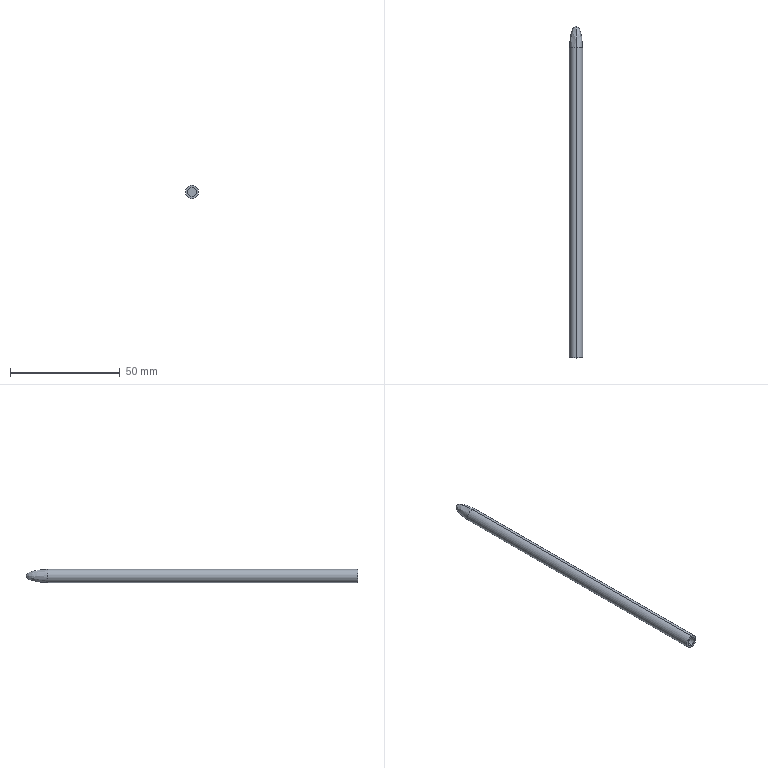Part | SolidWorks | features BaseBody 1 | 1 solid | 8 faces | box 6 x 151 x 6 mm | volume 2416 mm3 | cylinder 4 | plane 2 | spline 2 | commonest cylinder face diameters 4 x2 6 x2
STEP:
#1=CARTESIAN_POINT('',(0.,62.199,-3.));
#2=VERTEX_POINT('',#1);
#3=CARTESIAN_POINT('',(0.,62.199,3.));
#4=VERTEX_POINT('',#3);
#5=CARTESIAN_POINT('',(0.,62.199,0.));
#6=DIRECTION('',(0.,-1.,0.));
#7=DIRECTION('',(0.,0.,-1.));
#8=AXIS2_PLACEMENT_3D('',#5,#6,#7);
#9=CIRCLE('',#8,3.);
#10=EDGE_CURVE('',#2,#4,#9,.T.);
#11=ORIENTED_EDGE('',*,*,#10,.T.);
#12=CARTESIAN_POINT('',(0.,-78.801,3.));
#13=VERTEX_POINT('',#12);
#14=CARTESIAN_POINT('',(0.,0.,3.));
#15=DIRECTION('',(0.,-1.,0.));
#16=VECTOR('',#15,1000.);
#17=LINE('',#14,#16);
#18=EDGE_CURVE('',#4,#13,#17,.T.);
#19=ORIENTED_EDGE('',*,*,#18,.T.);
#20=CARTESIAN_POINT('',(0.,-78.801,-3.));
#21=VERTEX_POINT('',#20);
#22=CARTESIAN_POINT('',(0.,-78.801,0.));
#23=DIRECTION('',(0.,1.,0.));
#24=DIRECTION('',(0.,0.,-1.));
#25=AXIS2_PLACEMENT_3D('',#22,#23,#24);
#26=CIRCLE('',#25,3.);
#27=EDGE_CURVE('',#13,#21,#26,.T.);
#28=ORIENTED_EDGE('',*,*,#27,.T.);
#29=CARTESIAN_POINT('',(0.,0.,-3.));
#30=DIRECTION('',(0.,-1.,0.));
#31=VECTOR('',#30,1000.);
#32=LINE('',#29,#31);
#33=EDGE_CURVE('',#2,#21,#32,.T.);
#34=ORIENTED_EDGE('',*,*,#33,.F.);
#35=EDGE_LOOP('',(#11,#19,#28,#34));
#36=FACE_OUTER_BOUND('',#35,.T.);
#37=CARTESIAN_POINT('',(0.,0.,0.));
#38=DIRECTION('',(0.,-1.,0.));
#39=DIRECTION('',(0.,0.,-1.));
#40=AXIS2_PLACEMENT_3D('',#37,#38,#39);
#41=CYLINDRICAL_SURFACE('',#40,3.);
#42=ADVANCED_FACE('',(#36),#41,.T.);
#43=CARTESIAN_POINT('',(0.,61.199,2.));
#44=VERTEX_POINT('',#43);
#45=CARTESIAN_POINT('',(0.,61.199,-2.));
#46=VERTEX_POINT('',#45);
#47=CARTESIAN_POINT('',(0.,61.199,0.));
#48=DIRECTION('',(0.,-1.,0.));
#49=DIRECTION('',(0.,0.,-1.));
#50=AXIS2_PLACEMENT_3D('',#47,#48,#49);
#51=CIRCLE('',#50,2.);
#52=EDGE_CURVE('',#44,#46,#51,.T.);
#53=ORIENTED_EDGE('',*,*,#52,.F.);
#54=CARTESIAN_POINT('',(0.,-78.801,2.));
#55=VERTEX_POINT('',#54);
#56=CARTESIAN_POINT('',(0.,0.,2.));
#57=DIRECTION('',(0.,-1.,0.));
#58=VECTOR('',#57,1000.);
#59=LINE('',#56,#58);
#60=EDGE_CURVE('',#44,#55,#59,.T.);
#61=ORIENTED_EDGE('',*,*,#60,.T.);
#62=CARTESIAN_POINT('',(0.,-78.801,-2.));
#63=VERTEX_POINT('',#62);
#64=CARTESIAN_POINT('',(0.,-78.801,0.));
#65=DIRECTION('',(0.,-1.,0.));
#66=DIRECTION('',(0.,0.,-1.));
#67=AXIS2_PLACEMENT_3D('',#64,#65,#66);
#68=CIRCLE('',#67,2.);
#69=EDGE_CURVE('',#55,#63,#68,.T.);
#70=ORIENTED_EDGE('',*,*,#69,.T.);
#71=CARTESIAN_POINT('',(0.,0.,-2.));
#72=DIRECTION('',(0.,-1.,0.));
#73=VECTOR('',#72,1000.);
#74=LINE('',#71,#73);
#75=EDGE_CURVE('',#46,#63,#74,.T.);
#76=ORIENTED_EDGE('',*,*,#75,.F.);
#77=EDGE_LOOP('',(#53,#61,#70,#76));
#78=FACE_OUTER_BOUND('',#77,.T.);
#79=CARTESIAN_POINT('',(0.,0.,0.));
#80=DIRECTION('',(0.,-1.,0.));
#81=DIRECTION('',(0.,0.,-1.));
#82=AXIS2_PLACEMENT_3D('',#79,#80,#81);
#83=CYLINDRICAL_SURFACE('',#82,2.);
#84=ADVANCED_FACE('',(#78),#83,.F.);
#85=ORIENTED_EDGE('',*,*,#18,.F.);
#86=CARTESIAN_POINT('',(0.,62.199,0.));
#87=DIRECTION('',(0.,-1.,0.));
#88=DIRECTION('',(0.,0.,-1.));
#89=AXIS2_PLACEMENT_3D('',#86,#87,#88);
#90=CIRCLE('',#89,3.);
#91=EDGE_CURVE('',#4,#2,#90,.T.);
#92=ORIENTED_EDGE('',*,*,#91,.T.);
#93=ORIENTED_EDGE('',*,*,#33,.T.);
#94=CARTESIAN_POINT('',(0.,-78.801,0.));
#95=DIRECTION('',(0.,1.,0.));
#96=DIRECTION('',(0.,0.,-1.));
#97=AXIS2_PLACEMENT_3D('',#94,#95,#96);
#98=CIRCLE('',#97,3.);
#99=EDGE_CURVE('',#21,#13,#98,.T.);
#100=ORIENTED_EDGE('',*,*,#99,.T.);
#101=EDGE_LOOP('',(#85,#92,#93,#100));
#102=FACE_OUTER_BOUND('',#101,.T.);
#103=CARTESIAN_POINT('',(0.,0.,0.));
#104=DIRECTION('',(0.,-1.,0.));
#105=DIRECTION('',(0.,0.,-1.));
#106=AXIS2_PLACEMENT_3D('',#103,#104,#105);
#107=CYLINDRICAL_SURFACE('',#106,3.);
#108=ADVANCED_FACE('',(#102),#107,.T.);
#109=ORIENTED_EDGE('',*,*,#99,.F.);
#110=ORIENTED_EDGE('',*,*,#27,.F.);
#111=EDGE_LOOP('',(#109,#110));
#112=FACE_OUTER_BOUND('',#111,.T.);
#113=CARTESIAN_POINT('',(0.,-78.801,0.));
#114=DIRECTION('',(0.,-1.,0.));
#115=DIRECTION('',(0.,0.,-1.));
#116=AXIS2_PLACEMENT_3D('',#113,#114,#115);
#117=CIRCLE('',#116,2.);
#118=EDGE_CURVE('',#63,#55,#117,.T.);
#119=ORIENTED_EDGE('',*,*,#118,.F.);
#120=ORIENTED_EDGE('',*,*,#69,.F.);
#121=EDGE_LOOP('',(#119,#120));
#122=FACE_BOUND('',#121,.T.);
#123=CARTESIAN_POINT('',(-2.,-78.801,0.));
#124=DIRECTION('',(0.,1.,0.));
#125=DIRECTION('',(0.,0.,1.));
#126=AXIS2_PLACEMENT_3D('',#123,#124,#125);
#127=PLANE('',#126);
#128=ADVANCED_FACE('',(#112,#122),#127,.F.);
#129=CARTESIAN_POINT('',(0.,72.199,0.));
#130=VERTEX_POINT('',#129);
#131=CARTESIAN_POINT('',(0.,72.199,0.));
#132=CARTESIAN_POINT('',(0.,72.199,1.757));
#133=CARTESIAN_POINT('',(0.,68.057,3.));
#134=CARTESIAN_POINT('',(0.,62.199,3.));
#135=(BOUNDED_CURVE()B_SPLINE_CURVE(3,(#131,#132,#133,#134),.UNSPECIFIED.,.F.,.F.)B_SPLINE_CURVE_WITH_KNOTS((4,4),(0.,1.),.UNSPECIFIED.)CURVE()GEOMETRIC_REPRESENTATION_ITEM()RATIONAL_B_SPLINE_CURVE((1.,0.8047,0.8047,1.))REPRESENTATION_ITEM(''));
#136=EDGE_CURVE('',#130,#4,#135,.T.);
#137=ORIENTED_EDGE('',*,*,#136,.T.);
#138=ORIENTED_EDGE('',*,*,#10,.F.);
#139=CARTESIAN_POINT('',(0.,62.199,-3.));
#140=CARTESIAN_POINT('',(0.,68.057,-3.));
#141=CARTESIAN_POINT('',(0.,72.199,-1.757));
#142=CARTESIAN_POINT('',(0.,72.199,0.));
#143=(BOUNDED_CURVE()B_SPLINE_CURVE(3,(#139,#140,#141,#142),.UNSPECIFIED.,.F.,.T.)B_SPLINE_CURVE_WITH_KNOTS((4,4),(0.,1.),.UNSPECIFIED.)CURVE()GEOMETRIC_REPRESENTATION_ITEM()RATIONAL_B_SPLINE_CURVE((1.,0.8047,0.8047,1.))REPRESENTATION_ITEM(''));
#144=EDGE_CURVE('',#2,#130,#143,.T.);
#145=ORIENTED_EDGE('',*,*,#144,.T.);
#146=EDGE_LOOP('',(#137,#138,#145));
#147=FACE_OUTER_BOUND('',#146,.T.);
#148=CARTESIAN_POINT('',(0.,72.199,0.));
#149=CARTESIAN_POINT('',(0.,72.199,0.));
#150=CARTESIAN_POINT('',(0.,72.199,0.));
#151=CARTESIAN_POINT('',(0.,72.199,0.));
#152=CARTESIAN_POINT('',(0.,72.199,1.757));
#153=CARTESIAN_POINT('',(3.515,72.199,1.757));
#154=CARTESIAN_POINT('',(3.515,72.199,-1.757));
#155=CARTESIAN_POINT('',(0.,72.199,-1.757));
#156=CARTESIAN_POINT('',(0.,68.057,3.));
#157=CARTESIAN_POINT('',(6.,68.057,3.));
#158=CARTESIAN_POINT('',(6.,68.057,-3.));
#159=CARTESIAN_POINT('',(0.,68.057,-3.));
#160=CARTESIAN_POINT('',(0.,62.199,3.));
#161=CARTESIAN_POINT('',(6.,62.199,3.));
#162=CARTESIAN_POINT('',(6.,62.199,-3.));
#163=CARTESIAN_POINT('',(0.,62.199,-3.));
#164=(BOUNDED_SURFACE()B_SPLINE_SURFACE(3,3,((#148,#149,#150,#151),(#152,#153,#154,#155),(#156,#157,#158,#159),(#160,#161,#162,#163)),.UNSPECIFIED.,.F.,.F.,.F.)B_SPLINE_SURFACE_WITH_KNOTS((4,4),(4,4),(0.,1.),(0.,1.),.UNSPECIFIED.)GEOMETRIC_REPRESENTATION_ITEM()RATIONAL_B_SPLINE_SURFACE(((1.,0.3333,0.3333,1.),(0.8047,0.2682,0.2682,0.8047),(0.8047,0.2682,0.2682,0.8047),(1.,0.3333,0.3333,1.)))REPRESENTATION_ITEM('')SURFACE());
#165=ADVANCED_FACE('',(#147),#164,.T.);
#166=ORIENTED_EDGE('',*,*,#144,.F.);
#167=ORIENTED_EDGE('',*,*,#91,.F.);
#168=ORIENTED_EDGE('',*,*,#136,.F.);
#169=EDGE_LOOP('',(#166,#167,#168));
#170=FACE_OUTER_BOUND('',#169,.T.);
#171=CARTESIAN_POINT('',(0.,72.199,0.));
#172=CARTESIAN_POINT('',(0.,72.199,0.));
#173=CARTESIAN_POINT('',(0.,72.199,0.));
#174=CARTESIAN_POINT('',(0.,72.199,0.));
#175=CARTESIAN_POINT('',(0.,72.199,-1.757));
#176=CARTESIAN_POINT('',(-3.515,72.199,-1.757));
#177=CARTESIAN_POINT('',(-3.515,72.199,1.757));
#178=CARTESIAN_POINT('',(0.,72.199,1.757));
#179=CARTESIAN_POINT('',(0.,68.057,-3.));
#180=CARTESIAN_POINT('',(-6.,68.057,-3.));
#181=CARTESIAN_POINT('',(-6.,68.057,3.));
#182=CARTESIAN_POINT('',(0.,68.057,3.));
#183=CARTESIAN_POINT('',(0.,62.199,-3.));
#184=CARTESIAN_POINT('',(-6.,62.199,-3.));
#185=CARTESIAN_POINT('',(-6.,62.199,3.));
#186=CARTESIAN_POINT('',(0.,62.199,3.));
#187=(BOUNDED_SURFACE()B_SPLINE_SURFACE(3,3,((#171,#172,#173,#174),(#175,#176,#177,#178),(#179,#180,#181,#182),(#183,#184,#185,#186)),.UNSPECIFIED.,.F.,.F.,.T.)B_SPLINE_SURFACE_WITH_KNOTS((4,4),(4,4),(0.,1.),(0.,1.),.UNSPECIFIED.)GEOMETRIC_REPRESENTATION_ITEM()RATIONAL_B_SPLINE_SURFACE(((1.,0.3333,0.3333,1.),(0.8047,0.2682,0.2682,0.8047),(0.8047,0.2682,0.2682,0.8047),(1.,0.3333,0.3333,1.)))REPRESENTATION_ITEM('')SURFACE());
#188=ADVANCED_FACE('',(#170),#187,.T.);
#189=ORIENTED_EDGE('',*,*,#60,.F.);
#190=CARTESIAN_POINT('',(0.,61.199,0.));
#191=DIRECTION('',(0.,-1.,0.));
#192=DIRECTION('',(0.,0.,-1.));
#193=AXIS2_PLACEMENT_3D('',#190,#191,#192);
#194=CIRCLE('',#193,2.);
#195=EDGE_CURVE('',#46,#44,#194,.T.);
#196=ORIENTED_EDGE('',*,*,#195,.F.);
#197=ORIENTED_EDGE('',*,*,#75,.T.);
#198=ORIENTED_EDGE('',*,*,#118,.T.);
#199=EDGE_LOOP('',(#189,#196,#197,#198));
#200=FACE_OUTER_BOUND('',#199,.T.);
#201=CARTESIAN_POINT('',(0.,0.,0.));
#202=DIRECTION('',(0.,-1.,0.));
#203=DIRECTION('',(0.,0.,-1.));
#204=AXIS2_PLACEMENT_3D('',#201,#202,#203);
#205=CYLINDRICAL_SURFACE('',#204,2.);
#206=ADVANCED_FACE('',(#200),#205,.F.);
#207=ORIENTED_EDGE('',*,*,#195,.T.);
#208=ORIENTED_EDGE('',*,*,#52,.T.);
#209=EDGE_LOOP('',(#207,#208));
#210=FACE_OUTER_BOUND('',#209,.T.);
#211=CARTESIAN_POINT('',(0.,61.199,0.));
#212=DIRECTION('',(0.,1.,0.));
#213=DIRECTION('',(0.,0.,1.));
#214=AXIS2_PLACEMENT_3D('',#211,#212,#213);
#215=PLANE('',#214);
#216=ADVANCED_FACE('',(#210),#215,.F.);
#217=CLOSED_SHELL('',(#42,#84,#108,#128,#165,#188,#206,#216));
#218=MANIFOLD_SOLID_BREP('',#217);
#219=CARTESIAN_POINT('',(0.,0.,0.));
#220=DIRECTION('',(0.,0.,1.));
#221=DIRECTION('',(1.,0.,0.));
#222=AXIS2_PLACEMENT_3D('',#219,#220,#221);
#223=(LENGTH_UNIT()NAMED_UNIT(*)SI_UNIT(.MILLI.,.METRE.));
#224=UNCERTAINTY_MEASURE_WITH_UNIT(LENGTH_MEASURE(0.00001),#223,'','');
#225=(NAMED_UNIT(*)PLANE_ANGLE_UNIT()SI_UNIT($,.RADIAN.));
#226=(NAMED_UNIT(*)SI_UNIT($,.STERADIAN.)SOLID_ANGLE_UNIT());
#227=(GEOMETRIC_REPRESENTATION_CONTEXT(3)GLOBAL_UNCERTAINTY_ASSIGNED_CONTEXT((#224))GLOBAL_UNIT_ASSIGNED_CONTEXT((#223,#225,#226))REPRESENTATION_CONTEXT('',''));
#228=ADVANCED_BREP_SHAPE_REPRESENTATION('',(#218,#222),#227);